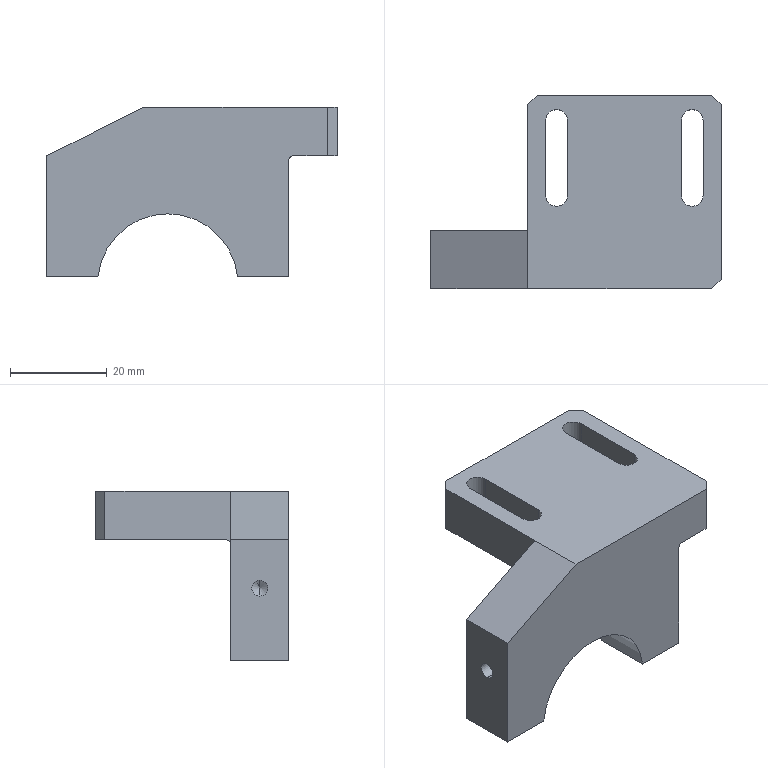NC program | NX | posted with a generic post | part box 60 x 40 x 35 mm
Lines 1 to 1065 of 5234:
N10 G17 G21 G94 G90
(FIXED_CONTOUR , TOOL : D10)
N12 T15 M6
N14 G54
N16 G17 G0 G90 X-10.456 Y25.201 S9500 M3
N18 G43 Z30. H15
N20 Z10.93
N22 G94 G1 X-11.051 Z10.828 F2500.
N24 X-11.629 Y25.2 Z10.655
N26 X-12.183 Z10.414
N28 X-12.703 Z10.107
N30 X-13.183 Z9.74
N32 X-13.614 Y25.199 Z9.318
N34 X-13.992 Z8.847
N36 X-14.31 Z8.334
N38 X-14.564 Z7.786
N40 X-14.75 Z7.212
N42 X-14.866 Z6.619
N44 X-14.909 Z6.017
N46 X-14.88 Z5.414
N48 X-14.302 Z0.162
N50 X-14.194 Z-0.622
N52 X-14.145 Z-0.964
N54 X-14.067 Z-1.344
N56 X-13.911 Z-2.063
N58 X-13.666 Z-2.884
N60 X-13.598 Z-3.111
N62 X-13.285 Y25.2 Z-3.941
N64 X-13.129 Z-4.298
N66 X-12.817 Z-4.974
N68 X-12.504 Z-5.542
N70 X-12.191 Z-6.079
N72 X-11.879 Z-6.555
N74 X-11.566 Z-7.
N76 X-11.253 Z-7.408
N78 X-10.941 Y25.201 Z-7.792
N80 X-10.628 Z-8.144
N82 X-10.315 Z-8.487
N84 X-9.69 Z-9.093
N86 X-9.377 Z-9.365
N88 X-9.065 Z-9.627
N90 X-8.752 Y25.202 Z-9.882
N92 X-8.127 Z-10.331
N94 X-7.814 Z-10.542
N96 X-7.501 Z-10.734
N98 X-6.876 Z-11.1
N100 X-6.251 Y25.203 Z-11.423
N102 X-5.625 Z-11.702
N104 X-5. Z-11.956
N106 X-4.839 Z-11.9
N108 X-4.375 Z-11.702
N110 X-3.749 Y25.204 Z-11.423
N112 X-3.124 Z-11.1
N114 X-2.499 Z-10.734
N116 X-2.186 Z-10.542
N118 X-1.874 Y25.205 Z-10.332
N120 X-1.248 Z-9.882
N122 X-0.936 Z-9.627
N124 X-0.623 Z-9.365
N126 X-0.31 Z-9.094
N128 X0.315 Y25.206 Z-8.487
N130 X0.628 Z-8.144
N132 X0.94 Z-7.793
N134 X1.253 Z-7.408
N136 X1.566 Z-7.001
N138 X1.878 Z-6.555
N140 X2.191 Z-6.079
N142 X2.504 Z-5.543
N144 X2.816 Y25.207 Z-4.975
N146 X3.129 Z-4.299
N148 X3.285 Z-3.942
N150 X3.598 Z-3.112
N152 X3.84 Z-2.302
N154 X3.91 Z-2.064
N156 X4.067 Z-1.345
N158 X4.145 Z-0.967
N160 X4.223 Z-0.41
N162 X4.301 Z0.176
N164 X4.874 Y25.208 Z5.416
N166 X4.873 Y24.908 Z5.419
N168 X4.301 Y24.907 Z0.181
N170 X4.223 Z-0.407
N172 X4.145 Z-0.963
N174 X4.067 Z-1.343
N176 X3.91 Z-2.063
N178 X3.754 Z-2.593
N180 X3.598 Z-3.111
N182 X3.285 Z-3.941
N184 X3.129 Z-4.299
N186 X2.816 Z-4.974
N188 X2.503 Y24.906 Z-5.543
N190 X2.191 Z-6.079
N192 X1.878 Z-6.555
N194 X1.566 Z-7.
N196 X1.253 Z-7.408
N198 X0.94 Z-7.793
N200 X0.628 Z-8.144
N202 X0.315 Z-8.487
N204 X-0.31 Y24.905 Z-9.093
N206 X-0.623 Z-9.365
N208 X-0.936 Z-9.627
N210 X-1.248 Z-9.882
N212 X-1.874 Z-10.332
N214 X-2.186 Y24.904 Z-10.542
N216 X-2.499 Z-10.734
N218 X-3.124 Z-11.1
N220 X-3.75 Z-11.423
N222 X-4.375 Y24.903 Z-11.702
N224 X-4.85 Z-11.905
N226 X-5. Z-11.956
N228 X-5.625 Z-11.702
N230 X-6.251 Z-11.423
N232 X-6.876 Y24.902 Z-11.1
N234 X-7.501 Z-10.734
N236 X-7.814 Z-10.542
N238 X-8.127 Z-10.331
N240 X-8.752 Z-9.882
N242 X-9.065 Y24.901 Z-9.626
N244 X-9.377 Z-9.365
N246 X-9.69 Z-9.093
N248 X-10.315 Z-8.486
N250 X-10.628 Z-8.143
N252 X-10.941 Z-7.792
N254 X-11.253 Y24.9 Z-7.408
N256 X-11.566 Z-7.
N258 X-11.879 Z-6.555
N260 X-12.191 Z-6.078
N262 X-12.504 Z-5.542
N264 X-12.817 Z-4.973
N266 X-13.129 Z-4.298
N268 X-13.285 Z-3.94
N270 X-13.598 Y24.899 Z-3.11
N272 X-13.754 Z-2.592
N274 X-13.911 Z-2.062
N276 X-14.067 Z-1.342
N278 X-14.145 Z-0.961
N280 X-14.223 Z-0.408
N282 X-14.302 Z0.169
N284 X-14.88 Z5.416
N286 X-14.881 Y24.599 Z5.419
N288 X-14.302 Z0.173
N290 X-14.223 Z-0.407
N292 X-14.145 Z-0.961
N294 X-14.067 Z-1.343
N296 X-13.911 Z-2.062
N298 X-13.754 Z-2.592
N300 X-13.598 Z-3.11
N302 X-13.285 Y24.6 Z-3.94
N304 X-13.129 Z-4.298
N306 X-12.817 Z-4.973
N308 X-12.504 Z-5.542
N310 X-12.191 Z-6.078
N312 X-11.879 Z-6.555
N314 X-11.566 Z-7.
N316 X-11.253 Z-7.408
N318 X-10.941 Y24.601 Z-7.792
N320 X-10.628 Z-8.143
N322 X-10.315 Z-8.486
N324 X-9.69 Z-9.093
N326 X-9.377 Z-9.365
N328 X-9.065 Z-9.626
N330 X-8.752 Y24.602 Z-9.882
N332 X-8.127 Z-10.331
N334 X-7.814 Z-10.542
N336 X-7.501 Z-10.734
N338 X-6.876 Z-11.1
N340 X-6.251 Y24.603 Z-11.423
N342 X-5.625 Z-11.702
N344 X-5. Z-11.956
N346 X-4.85 Z-11.905
N348 X-4.375 Z-11.702
N350 X-3.75 Y24.604 Z-11.423
N352 X-3.124 Z-11.1
N354 X-2.499 Z-10.734
N356 X-2.186 Z-10.542
N358 X-1.874 Y24.605 Z-10.332
N360 X-1.248 Z-9.882
N362 X-0.936 Z-9.627
N364 X-0.623 Z-9.365
N366 X-0.31 Z-9.093
N368 X0.315 Y24.606 Z-8.487
N370 X0.628 Z-8.144
N372 X0.94 Z-7.793
N374 X1.253 Z-7.408
N376 X1.566 Z-7.
N378 X1.878 Z-6.555
N380 X2.191 Z-6.079
N382 X2.503 Y24.607 Z-5.543
N384 X2.816 Z-4.974
N386 X3.129 Z-4.299
N388 X3.285 Z-3.941
N390 X3.598 Z-3.111
N392 X3.754 Z-2.593
N394 X3.91 Z-2.063
N396 X4.067 Z-1.344
N398 X4.145 Z-0.963
N400 X4.223 Z-0.407
N402 X4.301 Z0.181
N404 X4.874 Y24.608 Z5.421
N406 X4.875 Y24.308 Z5.423
N408 X4.301 Y24.307 Z0.18
N410 X4.223 Z-0.407
N412 X4.145 Z-0.963
N414 X4.067 Z-1.344
N416 X3.91 Z-2.063
N418 X3.754 Z-2.593
N420 X3.598 Z-3.111
N422 X3.285 Z-3.941
N424 X3.129 Z-4.299
N426 X2.816 Z-4.974
N428 X2.503 Z-5.543
N430 X2.191 Y24.306 Z-6.079
N432 X1.878 Z-6.555
N434 X1.566 Z-7.
N436 X1.253 Z-7.408
N438 X0.94 Z-7.793
N440 X0.628 Z-8.144
N442 X0.315 Z-8.487
N444 X-0.31 Y24.305 Z-9.093
N446 X-0.623 Z-9.365
N448 X-0.936 Z-9.627
N450 X-1.248 Z-9.882
N452 X-1.874 Z-10.332
N454 X-2.186 Y24.304 Z-10.542
N456 X-2.499 Z-10.734
N458 X-3.124 Z-11.1
N460 X-3.75 Z-11.423
N462 X-4.375 Z-11.702
N464 X-4.85 Y24.303 Z-11.905
N466 X-5. Z-11.956
N468 X-5.625 Z-11.702
N470 X-6.251 Z-11.423
N472 X-6.876 Y24.302 Z-11.1
N474 X-7.501 Z-10.734
N476 X-7.814 Z-10.542
N478 X-8.127 Z-10.331
N480 X-8.752 Z-9.882
N482 X-9.065 Y24.301 Z-9.626
N484 X-9.377 Z-9.365
N486 X-9.69 Z-9.093
N488 X-10.315 Z-8.486
N490 X-10.628 Z-8.143
N492 X-10.941 Z-7.792
N494 X-11.253 Z-7.408
N496 X-11.566 Y24.3 Z-7.
N498 X-11.879 Z-6.555
N500 X-12.191 Z-6.078
N502 X-12.504 Z-5.542
N504 X-12.817 Z-4.973
N506 X-13.129 Z-4.298
N508 X-13.285 Z-3.94
N510 X-13.598 Y24.299 Z-3.11
N512 X-13.754 Z-2.592
N514 X-13.911 Z-2.062
N516 X-14.067 Z-1.343
N518 X-14.145 Z-0.961
N520 X-14.223 Z-0.406
N522 X-14.302 Z0.176
N524 X-14.881 Z5.421
N526 X-14.882 Y23.999 Z5.423
N528 X-14.302 Z0.17
N530 X-14.223 Z-0.408
N532 X-14.145 Z-0.962
N534 X-14.067 Z-1.343
N536 X-13.911 Z-2.062
N538 X-13.754 Z-2.592
N540 X-13.598 Z-3.11
N542 X-13.285 Y24. Z-3.94
N544 X-13.129 Z-4.298
N546 X-12.817 Z-4.973
N548 X-12.504 Z-5.542
N550 X-12.191 Z-6.078
N552 X-11.879 Z-6.555
N554 X-11.566 Z-7.
N556 X-11.253 Y24.001 Z-7.408
N558 X-10.941 Z-7.792
N560 X-10.628 Z-8.143
N562 X-10.315 Z-8.486
N564 X-9.69 Z-9.093
N566 X-9.377 Z-9.365
N568 X-9.065 Z-9.626
N570 X-8.752 Y24.002 Z-9.882
N572 X-8.127 Z-10.331
N574 X-7.814 Z-10.542
N576 X-7.501 Z-10.734
N578 X-6.876 Z-11.1
N580 X-6.251 Y24.003 Z-11.423
N582 X-5.625 Z-11.702
N584 X-5. Z-11.956
N586 X-4.85 Z-11.905
N588 X-4.375 Y24.004 Z-11.702
N590 X-3.75 Z-11.423
N592 X-3.124 Z-11.1
N594 X-2.499 Z-10.734
N596 X-2.186 Z-10.542
N598 X-1.874 Y24.005 Z-10.332
N600 X-1.248 Z-9.882
N602 X-0.936 Z-9.627
N604 X-0.623 Z-9.365
N606 X-0.31 Z-9.093
N608 X0.315 Y24.006 Z-8.487
N610 X0.628 Z-8.144
N612 X0.94 Z-7.793
N614 X1.253 Z-7.408
N616 X1.566 Z-7.
N618 X1.878 Z-6.555
N620 X2.191 Z-6.079
N622 X2.503 Y24.007 Z-5.543
N624 X2.816 Z-4.974
N626 X3.129 Z-4.299
N628 X3.285 Z-3.941
N630 X3.598 Z-3.111
N632 X3.754 Z-2.593
N634 X3.91 Z-2.063
N636 X4.067 Z-1.344
N638 X4.145 Z-0.963
N640 X4.265 Z-0.1
N642 X4.301 Z0.173
N644 X4.876 Y24.008 Z5.425
N646 X4.877 Y23.708 Z5.427
N648 X4.379 Y23.707 Z0.867
N650 X4.301 Z0.167
N652 X4.224 Z-0.4
N654 X4.145 Z-0.963
N656 X4.068 Z-1.339
N658 X3.91 Z-2.063
N660 X3.756 Z-2.586
N662 X3.598 Z-3.111
N664 X3.285 Z-3.941
N666 X3.129 Z-4.299
N668 X2.816 Z-4.974
N670 X2.503 Z-5.543
N672 X2.191 Y23.706 Z-6.079
N674 X1.878 Z-6.555
N676 X1.566 Z-7.
N678 X1.253 Z-7.408
N680 X0.94 Z-7.793
N682 X0.633 Z-8.138
N684 X0.315 Z-8.487
N686 X-0.31 Y23.705 Z-9.093
N688 X-0.623 Z-9.365
N690 X-0.936 Z-9.627
N692 X-1.248 Z-9.882
N694 X-1.874 Z-10.332
N696 X-2.186 Y23.704 Z-10.542
N698 X-2.499 Z-10.734
N700 X-3.124 Z-11.1
N702 X-3.75 Z-11.423
N704 X-4.375 Z-11.702
N706 X-4.85 Y23.703 Z-11.904
N708 X-5. Z-11.956
N710 X-5.625 Z-11.702
N712 X-6.251 Z-11.423
N714 X-6.876 Y23.702 Z-11.1
N716 X-7.501 Z-10.734
N718 X-7.814 Z-10.542
N720 X-8.127 Z-10.331
N722 X-8.752 Z-9.882
N724 X-9.065 Y23.701 Z-9.626
N726 X-9.377 Z-9.365
N728 X-9.69 Z-9.093
N730 X-10.315 Z-8.486
N732 X-10.628 Z-8.143
N734 X-10.941 Z-7.792
N736 X-11.253 Z-7.408
N738 X-11.566 Y23.7 Z-7.
N740 X-11.879 Z-6.555
N742 X-12.191 Z-6.078
N744 X-12.504 Z-5.542
N746 X-12.817 Z-4.973
N748 X-13.129 Z-4.298
N750 X-13.285 Z-3.94
N752 X-13.598 Z-3.11
N754 X-13.754 Y23.699 Z-2.592
N756 X-13.911 Z-2.062
N758 X-14.067 Z-1.343
N760 X-14.145 Z-0.963
N762 X-14.223 Z-0.411
N764 X-14.304 Z0.182
N766 X-14.883 Z5.426
N768 Y23.399 Z5.428
N770 X-14.341 Z0.498
N772 X-14.262 Z-0.132
N774 X-14.185 Z-0.69
N776 X-14.145 Z-0.963
N778 X-14.067 Z-1.343
N780 X-13.911 Z-2.062
N782 X-13.754 Z-2.592
N784 X-13.598 Y23.4 Z-3.11
N786 X-13.285 Z-3.94
N788 X-13.129 Z-4.298
N790 X-12.817 Z-4.973
N792 X-12.504 Z-5.542
N794 X-12.191 Z-6.078
N796 X-11.879 Z-6.555
N798 X-11.566 Z-7.
N800 X-11.253 Y23.401 Z-7.408
N802 X-10.941 Z-7.792
N804 X-10.628 Z-8.143
N806 X-10.315 Z-8.486
N808 X-9.69 Z-9.093
N810 X-9.377 Z-9.365
N812 X-9.065 Y23.402 Z-9.626
N814 X-8.752 Z-9.882
N816 X-8.127 Z-10.331
N818 X-7.814 Z-10.542
N820 X-7.501 Z-10.734
N822 X-6.876 Z-11.1
N824 X-6.251 Y23.403 Z-11.423
N826 X-5.625 Z-11.702
N828 X-5. Z-11.956
N830 X-4.85 Z-11.905
N832 X-4.375 Y23.404 Z-11.702
N834 X-3.75 Z-11.423
N836 X-3.124 Z-11.1
N838 X-2.499 Z-10.734
N840 X-2.186 Y23.405 Z-10.542
N842 X-1.874 Z-10.332
N844 X-1.248 Z-9.882
N846 X-0.936 Z-9.627
N848 X-0.623 Z-9.365
N850 X-0.31 Z-9.093
N852 X0.315 Y23.406 Z-8.487
N854 X0.628 Z-8.144
N856 X0.94 Z-7.793
N858 X1.253 Z-7.408
N860 X1.566 Z-7.
N862 X1.878 Z-6.555
N864 X2.191 Z-6.079
N866 X2.503 Y23.407 Z-5.543
N868 X2.816 Z-4.974
N870 X3.129 Z-4.299
N872 X3.285 Z-3.941
N874 X3.598 Z-3.111
N876 X3.754 Z-2.593
N878 X3.91 Z-2.064
N880 X4.067 Z-1.344
N882 X4.145 Z-0.963
N884 X4.301 Z0.155
N886 X4.379 Z0.855
N888 X4.632 Y23.408 Z3.171
N890 X4.755 Z4.259
N892 X4.878 Z5.429
N894 X4.879 Y23.108 Z5.432
N896 X4.636 Z3.123
N898 X4.301 Z0.143
N900 X4.145 Y23.107 Z-0.963
N902 X4.067 Z-1.344
N904 X3.91 Z-2.064
N906 X3.754 Z-2.593
N908 X3.598 Z-3.111
N910 X3.285 Z-3.941
N912 X3.129 Z-4.299
N914 X2.816 Z-4.974
N916 X2.503 Z-5.543
N918 X2.191 Z-6.079
N920 X1.878 Y23.106 Z-6.555
N922 X1.566 Z-7.
N924 X1.253 Z-7.408
N926 X0.94 Z-7.793
N928 X0.628 Z-8.144
N930 X0.315 Z-8.487
N932 X-0.31 Y23.105 Z-9.093
N934 X-0.623 Z-9.365
N936 X-0.936 Z-9.627
N938 X-1.248 Z-9.882
N940 X-1.874 Z-10.332
N942 X-2.186 Z-10.542
N944 X-2.499 Z-10.734
N946 X-3.124 Y23.104 Z-11.1
N948 X-3.75 Z-11.423
N950 X-4.375 Z-11.702
N952 X-4.85 Z-11.905
N954 X-5. Y23.103 Z-11.956
N956 X-5.625 Z-11.702
N958 X-6.251 Z-11.423
N960 X-6.876 Z-11.1
N962 X-7.501 Y23.102 Z-10.734
N964 X-7.814 Z-10.542
N966 X-8.127 Z-10.331
N968 X-8.752 Z-9.882
N970 X-9.058 Z-9.632
N972 X-9.377 Z-9.365
N974 X-9.69 Y23.101 Z-9.093
N976 X-10.315 Z-8.486
N978 X-10.628 Z-8.143
N980 X-10.941 Z-7.792
N982 X-11.253 Z-7.408
N984 X-11.566 Z-7.
N986 X-11.879 Y23.1 Z-6.555
N988 X-12.191 Z-6.078
N990 X-12.504 Z-5.542
N992 X-12.817 Z-4.973
N994 X-13.129 Z-4.298
N996 X-13.285 Z-3.94
N998 X-13.598 Z-3.11
N1000 X-13.752 Z-2.601
N1002 X-13.911 Z-2.062
N1004 X-14.067 Y23.099 Z-1.343
N1006 X-14.145 Z-0.963
N1008 X-14.223 Z-0.422
N1010 X-14.379 Z0.814
N1012 X-14.884 Z5.431
N1014 Y22.799 Z5.433
N1016 X-14.38 Z0.806
N1018 X-14.223 Z-0.428
N1020 X-14.145 Z-0.963
N1022 X-14.067 Y22.8 Z-1.343
N1024 X-13.911 Z-2.062
N1026 X-13.754 Z-2.592
N1028 X-13.598 Z-3.11
N1030 X-13.285 Z-3.94
N1032 X-13.129 Z-4.298
N1034 X-12.817 Z-4.973
N1036 X-12.504 Z-5.542
N1038 X-12.191 Z-6.078
N1040 X-11.879 Z-6.555
N1042 X-11.566 Y22.801 Z-7.
N1044 X-11.253 Z-7.408
N1046 X-10.941 Z-7.792
N1048 X-10.628 Z-8.143
N1050 X-10.315 Z-8.486
N1052 X-9.69 Z-9.093
N1054 X-9.377 Y22.802 Z-9.365
N1056 X-9.065 Z-9.626
N1058 X-8.752 Z-9.882
N1060 X-8.127 Z-10.331
N1062 X-7.814 Z-10.542
N1064 X-7.501 Z-10.734
N1066 X-6.876 Y22.803 Z-11.1
N1068 X-6.251 Z-11.423
N1070 X-5.625 Z-11.702
N1072 X-5. Z-11.956
N1074 X-4.85 Y22.804 Z-11.905
N1076 X-4.375 Z-11.702
N1078 X-3.75 Z-11.423
N1080 X-3.124 Z-11.1
N1082 X-2.499 Y22.805 Z-10.734
N1084 X-2.186 Z-10.542
N1086 X-1.874 Z-10.332
N1088 X-1.248 Z-9.882
N1090 X-0.936 Z-9.627
N1092 X-0.623 Z-9.365
N1094 X-0.31 Y22.806 Z-9.093
N1096 X0.315 Z-8.487
N1098 X0.628 Z-8.144
N1100 X0.94 Z-7.793
N1102 X1.253 Z-7.408
N1104 X1.566 Z-7.
N1106 X1.878 Z-6.555
N1108 X2.191 Y22.807 Z-6.079
N1110 X2.503 Z-5.543
N1112 X2.816 Z-4.974
N1114 X3.129 Z-4.299
N1116 X3.285 Z-3.941
N1118 X3.598 Z-3.111
N1120 X3.754 Z-2.593
N1122 X3.91 Z-2.064
N1124 X4.067 Z-1.345
N1126 X4.145 Z-0.963
N1128 X4.301 Y22.808 Z0.132
N1130 X4.629 Z3.045
N1132 X4.88 Z5.434
N1134 Y22.508 Z5.436
N1136 X4.63 Z3.036
N1138 X4.301 Z0.12
N1140 X4.145 Y22.507 Z-0.962
N1142 X4.067 Z-1.345
N1144 X3.91 Z-2.064
N1146 X3.754 Z-2.593
N1148 X3.598 Z-3.111
N1150 X3.285 Z-3.941
N1152 X3.129 Z-4.299
N1154 X2.816 Z-4.974
N1156 X2.503 Z-5.543
N1158 X2.191 Z-6.079
N1160 X1.878 Y22.506 Z-6.555
N1162 X1.566 Z-7.
N1164 X1.253 Z-7.408
N1166 X0.94 Z-7.793
N1168 X0.628 Z-8.144
N1170 X0.315 Z-8.487
N1172 X-0.31 Z-9.093
N1174 X-0.623 Y22.505 Z-9.365
N1176 X-0.936 Z-9.627
N1178 X-1.248 Z-9.882
N1180 X-1.874 Z-10.332
N1182 X-2.186 Z-10.542
N1184 X-2.499 Z-10.734
N1186 X-3.124 Y22.504 Z-11.1
N1188 X-3.75 Z-11.423
N1190 X-4.375 Z-11.702
N1192 X-4.85 Z-11.905
N1194 X-5. Y22.503 Z-11.956
N1196 X-5.625 Z-11.702
N1198 X-6.251 Z-11.423
N1200 X-6.876 Z-11.1
N1202 X-7.501 Y22.502 Z-10.734
N1204 X-7.814 Z-10.542
N1206 X-8.127 Z-10.331
N1208 X-8.752 Z-9.882
N1210 X-9.065 Z-9.626
N1212 X-9.377 Z-9.365
N1214 X-9.69 Y22.501 Z-9.093
N1216 X-10.315 Z-8.486
N1218 X-10.628 Z-8.143
N1220 X-10.941 Z-7.792
N1222 X-11.253 Z-7.408
N1224 X-11.566 Z-7.
N1226 X-11.879 Y22.5 Z-6.555
N1228 X-12.191 Z-6.078
N1230 X-12.504 Z-5.542
N1232 X-12.817 Z-4.973
N1234 X-13.129 Z-4.298
N1236 X-13.285 Z-3.94
N1238 X-13.598 Z-3.11
N1240 X-13.754 Z-2.592
N1242 X-13.911 Z-2.062
N1244 X-14.067 Z-1.344
N1246 X-14.145 Y22.499 Z-0.963
N1248 X-14.223 Z-0.433
N1250 X-14.38 Z0.788
N1252 X-14.885 Z5.436
N1254 X-14.886 Y22.199 Z5.438
N1256 X-14.38 Z0.777
N1258 X-14.223 Z-0.434
N1260 X-14.145 Z-0.963
N1262 X-14.067 Y22.2 Z-1.344
N1264 X-13.911 Z-2.062
N1266 X-13.754 Z-2.592
N1268 X-13.598 Z-3.11
N1270 X-13.285 Z-3.94
N1272 X-13.129 Z-4.298
N1274 X-12.817 Z-4.973
N1276 X-12.504 Z-5.542
N1278 X-12.191 Z-6.078
N1280 X-11.879 Z-6.555
N1282 X-11.566 Y22.201 Z-7.
N1284 X-11.253 Z-7.408
N1286 X-10.941 Z-7.792
N1288 X-10.628 Z-8.143
N1290 X-10.315 Z-8.486
N1292 X-9.69 Z-9.093
N1294 X-9.377 Y22.202 Z-9.365
N1296 X-9.065 Z-9.626
N1298 X-8.752 Z-9.882
N1300 X-8.127 Z-10.331
N1302 X-7.814 Z-10.542
N1304 X-7.501 Z-10.734
N1306 X-6.876 Y22.203 Z-11.1
N1308 X-6.251 Z-11.423
N1310 X-5.625 Z-11.702
N1312 X-5. Z-11.956
N1314 X-4.85 Y22.204 Z-11.905
N1316 X-4.375 Z-11.702
N1318 X-3.75 Z-11.423
N1320 X-3.124 Z-11.1
N1322 X-2.499 Y22.205 Z-10.734
N1324 X-2.186 Z-10.542
N1326 X-1.874 Z-10.332
N1328 X-1.248 Z-9.882
N1330 X-0.936 Z-9.627
N1332 X-0.623 Z-9.365
N1334 X-0.31 Y22.206 Z-9.093
N1336 X0.315 Z-8.487
N1338 X0.628 Z-8.144
N1340 X0.94 Z-7.793
N1342 X1.253 Z-7.408
N1344 X1.566 Z-7.
N1346 X1.878 Z-6.555
N1348 X2.191 Y22.207 Z-6.079
N1350 X2.503 Z-5.543
N1352 X2.816 Z-4.974
N1354 X3.129 Z-4.299
N1356 X3.285 Z-3.941
N1358 X3.598 Z-3.111
N1360 X3.754 Z-2.593
N1362 X3.91 Z-2.064
N1364 X4.067 Z-1.345
N1366 X4.145 Z-0.962
N1368 X4.301 Y22.208 Z0.108
N1370 X4.63 Z3.033
N1372 X4.881 Z5.438
N1374 X4.882 Y21.908 Z5.44
N1376 X4.631 Z3.03
N1378 X4.301 Z0.097
N1380 X4.145 Y21.907 Z-0.962
N1382 X4.067 Z-1.345
N1384 X3.91 Z-2.064
N1386 X3.754 Z-2.593
N1388 X3.598 Z-3.111
N1390 X3.285 Z-3.941
N1392 X3.129 Z-4.299
N1394 X2.816 Z-4.974
N1396 X2.503 Z-5.543
N1398 X2.191 Z-6.079
N1400 X1.878 Y21.906 Z-6.555
N1402 X1.566 Z-7.
N1404 X1.253 Z-7.408
N1406 X0.94 Z-7.793
N1408 X0.628 Z-8.144
N1410 X0.315 Z-8.487
N1412 X-0.31 Z-9.093
N1414 X-0.623 Y21.905 Z-9.365
N1416 X-0.936 Z-9.627
N1418 X-1.248 Z-9.882
N1420 X-1.874 Z-10.332
N1422 X-2.186 Z-10.542
N1424 X-2.499 Z-10.734
N1426 X-3.124 Y21.904 Z-11.1
N1428 X-3.75 Z-11.423
N1430 X-4.375 Z-11.702
N1432 X-4.85 Z-11.905
N1434 X-5. Y21.903 Z-11.956
N1436 X-5.625 Z-11.702
N1438 X-6.251 Z-11.423
N1440 X-6.876 Z-11.1
N1442 X-7.501 Y21.902 Z-10.734
N1444 X-7.814 Z-10.542
N1446 X-8.127 Z-10.331
N1448 X-8.752 Z-9.882
N1450 X-9.065 Z-9.626
N1452 X-9.377 Z-9.365
N1454 X-9.69 Y21.901 Z-9.093
N1456 X-10.315 Z-8.486
N1458 X-10.628 Z-8.143
N1460 X-10.941 Z-7.792
N1462 X-11.253 Z-7.408
N1464 X-11.566 Z-7.
N1466 X-11.879 Y21.9 Z-6.555
N1468 X-12.191 Z-6.078
N1470 X-12.504 Z-5.542
N1472 X-12.817 Z-4.973
N1474 X-13.129 Z-4.298
N1476 X-13.285 Z-3.94
N1478 X-13.598 Z-3.11
N1480 X-13.754 Z-2.592
N1482 X-13.911 Z-2.062
N1484 X-14.067 Z-1.344
N1486 X-14.145 Z-0.963
N1488 X-14.223 Y21.899 Z-0.434
N1490 X-14.38 Z0.768
N1492 X-14.886 Z5.44
N1494 X-14.887 Y21.599 Z5.443
N1496 X-14.38 Z0.761
N1498 X-14.223 Z-0.435
N1500 X-14.145 Y21.6 Z-0.964
N1502 X-14.067 Z-1.344
N1504 X-13.911 Z-2.063
N1506 X-13.754 Z-2.593
N1508 X-13.598 Z-3.11
N1510 X-13.285 Z-3.94
N1512 X-13.129 Z-4.299
N1514 X-12.817 Z-4.974
N1516 X-12.504 Z-5.542
N1518 X-12.191 Z-6.078
N1520 X-11.879 Y21.601 Z-6.555
N1522 X-11.566 Z-7.
N1524 X-11.253 Z-7.408
N1526 X-10.941 Z-7.792
N1528 X-10.628 Z-8.144
N1530 X-10.315 Z-8.486
N1532 X-9.69 Z-9.093
N1534 X-9.377 Y21.602 Z-9.365
N1536 X-9.065 Z-9.627
N1538 X-8.752 Z-9.882
N1540 X-8.127 Z-10.332
N1542 X-7.814 Z-10.542
N1544 X-7.501 Z-10.734
N1546 X-6.876 Y21.603 Z-11.1
N1548 X-6.251 Z-11.423
N1550 X-5.625 Z-11.702
N1552 X-5. Y21.604 Z-11.956
N1554 X-4.85 Z-11.905
N1556 X-4.375 Z-11.702
N1558 X-3.75 Z-11.423
N1560 X-3.124 Z-11.1
N1562 X-2.499 Y21.605 Z-10.734
N1564 X-2.186 Z-10.542
N1566 X-1.874 Z-10.332
N1568 X-1.248 Z-9.882
N1570 X-0.936 Z-9.627
N1572 X-0.623 Z-9.365
N1574 X-0.31 Y21.606 Z-9.094
N1576 X0.315 Z-8.487
N1578 X0.628 Z-8.144
N1580 X0.94 Z-7.793
N1582 X1.253 Z-7.408
N1584 X1.566 Z-7.
N1586 X1.878 Y21.607 Z-6.556
N1588 X2.191 Z-6.079
N1590 X2.503 Z-5.543
N1592 X2.816 Z-4.974
N1594 X3.129 Z-4.299
N1596 X3.285 Z-3.941
N1598 X3.598 Z-3.111
N1600 X3.754 Z-2.594
N1602 X3.91 Z-2.064
N1604 X4.095 Z-1.209
N1606 X4.145 Y21.608 Z-0.965
N1608 X4.301 Z0.084
N1610 X4.33 Z0.318
N1612 X4.54 Z2.186
N1614 X4.723 Z3.907
N1616 X4.883 Z5.443
N1618 X4.884 Y21.308 Z5.445
N1620 X4.419 Z1.076
N1622 X4.367 Z0.612
N1624 X4.301 Z0.07
N1626 X4.145 Z-0.968
N1628 X4.067 Z-1.347
N1630 X3.91 Y21.307 Z-2.065
N1632 X3.754 Z-2.594
N1634 X3.598 Z-3.112
N1636 X3.285 Z-3.941
N1638 X3.129 Z-4.3
N1640 X2.816 Z-4.975
N1642 X2.503 Z-5.543
N1644 X2.191 Z-6.079
N1646 X1.878 Z-6.556
N1648 X1.566 Y21.306 Z-7.
N1650 X1.253 Z-7.408
N1652 X0.94 Z-7.793
N1654 X0.628 Z-8.144
N1656 X0.315 Z-8.487
N1658 X-0.31 Z-9.094
N1660 X-0.623 Y21.305 Z-9.365
N1662 X-0.936 Z-9.627
N1664 X-1.248 Z-9.882
N1666 X-1.874 Z-10.332
N1668 X-2.186 Z-10.542
N1670 X-2.499 Z-10.734
N1672 X-3.124 Y21.304 Z-11.1
N1674 X-3.75 Z-11.423
N1676 X-4.375 Z-11.702
N1678 X-4.85 Z-11.905
N1680 X-5. Z-11.956
N1682 X-5.625 Y21.303 Z-11.702
N1684 X-6.251 Z-11.423
N1686 X-6.876 Z-11.1
N1688 X-7.501 Y21.302 Z-10.734
N1690 X-7.814 Z-10.542
N1692 X-8.127 Z-10.332
N1694 X-8.752 Z-9.882
N1696 X-9.065 Z-9.627
N1698 X-9.377 Z-9.365
N1700 X-9.69 Z-9.093
N1702 X-10.315 Y21.301 Z-8.487
N1704 X-10.628 Z-8.144
N1706 X-10.941 Z-7.792
N1708 X-11.253 Z-7.408
N1710 X-11.566 Z-7.
N1712 X-11.879 Z-6.555
N1714 X-12.191 Y21.3 Z-6.078
N1716 X-12.504 Z-5.543
N1718 X-12.817 Z-4.974
N1720 X-13.129 Z-4.299
N1722 X-13.285 Z-3.94
N1724 X-13.598 Z-3.111
N1726 X-13.754 Z-2.593
N1728 X-13.911 Z-2.064
N1730 X-14.067 Z-1.345
N1732 X-14.145 Z-0.965
N1734 X-14.223 Z-0.436
N1736 X-14.38 Y21.299 Z0.754
N1738 X-14.887 Z5.445
N1740 X-14.888 Y20.999 Z5.448
N1742 X-14.55 Y21. Z2.32
N1744 X-14.38 Z0.709
N1746 X-14.338 Z0.366
N1748 X-14.265 Z-0.188
N1750 X-14.145 Z-1.004
N1752 X-14.067 Z-1.374
N1754 X-13.911 Z-2.085
N1756 X-13.65 Z-2.961
N1758 X-13.598 Z-3.129
N1760 X-13.285 Z-3.958
N1762 X-13.129 Z-4.314
N1764 X-12.817 Z-4.989
N1766 X-12.504 Z-5.555
N1768 X-12.191 Y21.001 Z-6.09
N1770 X-11.879 Z-6.566
N1772 X-11.566 Z-7.01
N1774 X-11.253 Z-7.418
N1776 X-10.941 Z-7.801
N1778 X-10.628 Z-8.153
N1780 X-10.315 Z-8.495
N1782 X-9.69 Y21.002 Z-9.102
N1784 X-9.377 Z-9.373
N1786 X-9.065 Z-9.634
N1788 X-8.752 Z-9.889
N1790 X-8.127 Z-10.339
N1792 X-7.814 Z-10.548
N1794 X-7.501 Y21.003 Z-10.74
N1796 X-6.876 Z-11.106
N1798 X-6.251 Z-11.429
N1800 X-5.625 Z-11.707
N1802 X-5. Y21.004 Z-11.961
N1804 X-4.842 Z-11.907
N1806 X-4.375 Z-11.707
N1808 X-3.75 Z-11.429
N1810 X-3.124 Y21.005 Z-11.106
N1812 X-2.499 Z-10.74
N1814 X-2.186 Z-10.549
N1816 X-1.874 Z-10.339
N1818 X-1.248 Z-9.889
N1820 X-0.936 Z-9.634
N1822 X-0.623 Y21.006 Z-9.373
N1824 X-0.31 Z-9.102
N1826 X0.315 Z-8.495
N1828 X0.628 Z-8.153
N1830 X0.94 Z-7.802
N1832 X1.253 Z-7.418
N1834 X1.566 Y21.007 Z-7.01
N1836 X1.878 Z-6.567
N1838 X2.191 Z-6.09
N1840 X2.503 Z-5.556
N1842 X2.816 Z-4.989
N1844 X3.129 Z-4.314
N1846 X3.285 Z-3.959
N1848 X3.598 Z-3.129
N1850 X3.754 Y21.008 Z-2.616
N1852 X3.91 Z-2.086
N1854 X4.092 Z-1.26
N1856 X4.145 Z-1.003
N1858 X4.301 Z0.032
N1860 X4.379 Z0.673
N1862 X4.542 Z2.228
N1864 X4.885 Z5.447
N1866 X4.886 Y20.708 Z5.449
N1868 X4.784 Z4.494
N1870 X4.379 Z0.619
N1872 X4.301 Z-0.018
N1874 X4.207 Z-0.659
N1876 X4.145 Z-1.054
N1878 X4.067 Z-1.418
N1880 X3.91 Z-2.118
N1882 X3.723 Z-2.751
N1884 X3.598 Z-3.154
N1886 X3.285 Z-3.984
N1888 X3.129 Y20.707 Z-4.335
N1890 X2.816 Z-5.01
N1892 X2.503 Z-5.574
N1894 X2.191 Z-6.106
N1896 X1.878 Z-6.583
N1898 X1.566 Z-7.024
N1900 X1.253 Z-7.433
N1902 X0.94 Y20.706 Z-7.815
N1904 X0.565 Z-8.234
N1906 X0.315 Z-8.507
N1908 X-0.31 Z-9.114
N1910 X-0.623 Z-9.384
N1912 X-0.936 Z-9.645
N1914 X-1.248 Z-9.899
N1916 X-1.874 Y20.705 Z-10.349
N1918 X-2.186 Z-10.558
N1920 X-2.499 Z-10.75
N1922 X-3.124 Z-11.115
N1924 X-3.75 Y20.704 Z-11.438
N1926 X-4.375 Z-11.715
N1928 X-4.83 Z-11.91
N1930 X-5. Z-11.968
N1932 X-5.625 Z-11.715
N1934 X-6.251 Y20.703 Z-11.438
N1936 X-6.876 Z-11.115
N1938 X-7.501 Z-10.75
N1940 X-7.814 Z-10.558
N1942 X-8.127 Z-10.349
N1944 X-8.752 Y20.702 Z-9.899
N1946 X-9.065 Z-9.645
N1948 X-9.437 Z-9.331
N1950 X-9.69 Z-9.113
N1952 X-10.315 Z-8.507
N1954 X-10.628 Y20.701 Z-8.166
N1956 X-10.941 Z-7.814
N1958 X-11.253 Z-7.432
N1960 X-11.566 Z-7.024
N1962 X-11.879 Z-6.582
N1964 X-12.191 Z-6.106
N1966 X-12.504 Z-5.573
N1968 X-12.817 Y20.7 Z-5.01
N1970 X-13.129 Z-4.335
N1972 X-13.285 Z-3.983
N1974 X-13.598 Z-3.154
N1976 X-13.75 Z-2.661
N1978 X-13.911 Z-2.116
N1980 X-14.067 Z-1.416
N1982 X-14.145 Z-1.056
N1984 X-14.302 Z0.006
N1986 X-14.38 Z0.647
N1988 X-14.793 Z4.568
N1990 X-14.889 Z5.45
N1992 Y20.4 Z5.452
N1994 X-14.38 Z0.605
N1996 X-14.324 Z0.153
N1998 X-14.302 Z-0.049
N2000 X-14.168 Z-0.96
N2002 X-14.145 Z-1.1
N2004 X-14.077 Z-1.4
N2006 X-14.022 Z-1.656
N2008 X-13.911 Z-2.15
N2010 X-13.754 Z-2.679
N2012 X-13.598 Z-3.18
N2014 X-13.285 Z-4.01
N2016 X-13.129 Y20.401 Z-4.357
N2018 X-12.817 Z-5.03
N2020 X-12.504 Z-5.592
N2022 X-12.191 Z-6.122
N2024 X-11.879 Z-6.599
N2026 X-11.566 Z-7.039
N2028 X-11.253 Z-7.447
N2030 X-10.941 Z-7.828
N2032 X-10.628 Y20.402 Z-8.179
N2034 X-10.315 Z-8.519
N2036 X-9.69 Z-9.126
N2038 X-9.377 Z-9.395
N2040 X-9.065 Z-9.657
N2042 X-8.752 Z-9.91
N2044 X-8.127 Y20.403 Z-10.36
N2046 X-7.903 Z-10.509
N2048 X-7.68 Z-10.646
N2050 X-7.501 Z-10.76
N2052 X-6.876 Z-11.124
N2054 X-6.251 Y20.404 Z-11.447
N2056 X-5.625 Z-11.724
N2058 X-5. Z-11.977
N2060 X-4.825 Z-11.917
N2062 X-4.375 Z-11.725
N2064 X-3.75 Y20.405 Z-11.448
N2066 X-3.124 Z-11.125
N2068 X-2.499 Z-10.76
N2070 X-2.323 Z-10.648
N2072 X-2.098 Z-10.51
N2074 X-1.874 Z-10.36
N2076 X-1.248 Y20.406 Z-9.91
N2078 X-1.023 Z-9.728
N2080 X-0.799 Z-9.54
N2082 X-0.623 Z-9.395
N2084 X-0.31 Z-9.126
N2086 X0.315 Z-8.52
N2088 X0.628 Y20.407 Z-8.18
N2090 X0.94 Z-7.828
N2092 X1.253 Z-7.448
N2094 X1.566 Z-7.039
N2096 X1.878 Z-6.599
N2098 X2.191 Z-6.123
N2100 X2.503 Z-5.593
N2102 X2.816 Z-5.03
N2104 X3.129 Y20.408 Z-4.357
N2106 X3.285 Z-4.01
N2108 X3.598 Z-3.18
N2110 X3.754 Z-2.68
N2112 X3.91 Z-2.15
N2114 X4.067 Z-1.461
N2116 X4.145 Z-1.101
N2118 X4.223 Z-0.612
N2120 X4.301 Z-0.067
N2122 X4.323 Z0.126
N2124 X4.379 Z0.585
N2126 X4.887 Z5.451
N2128 X4.888 Y20.109 Z5.453